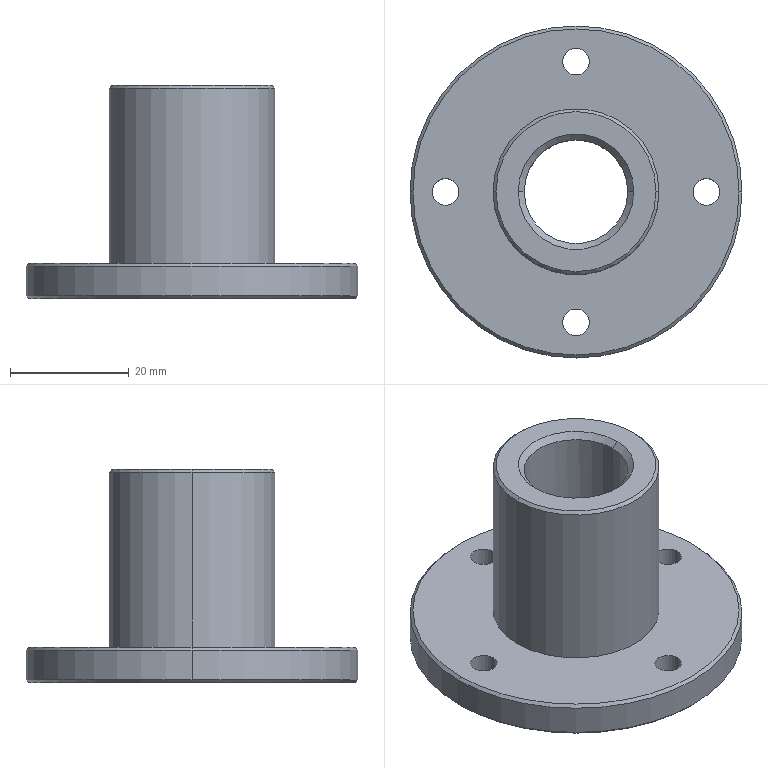Part | STEP file | adjusting nut 3 | 1 solid | 27 faces | box 56 x 56 x 36 mm | volume 24098 mm3 | cylinder 14 | cone 10 | plane 3 | commonest cylinder face diameters 4.5 x8 17.5 x2 28 x2 56 x2